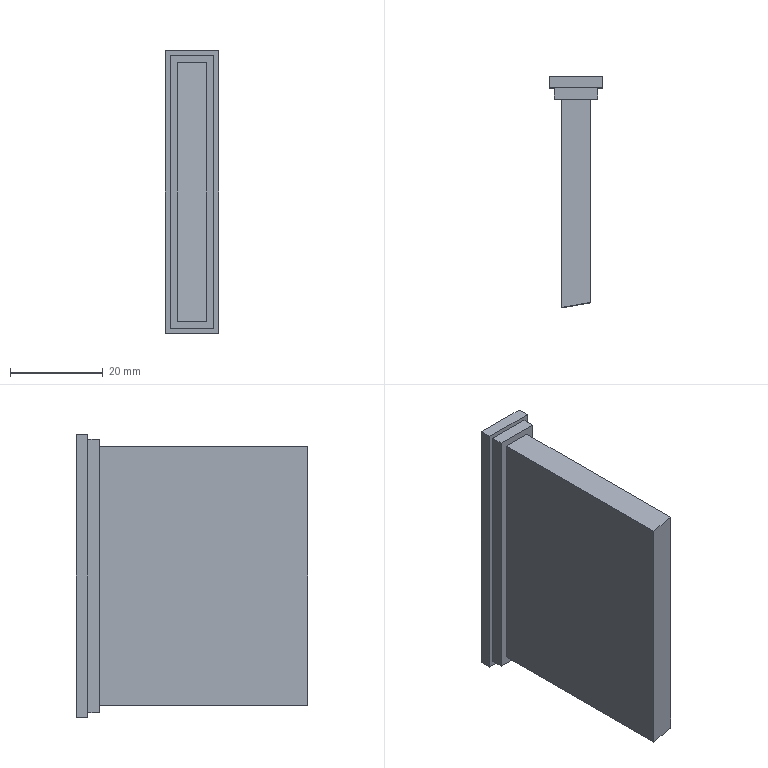Part | SolidWorks | features ICE 3, Extrusion 1 | 1 solid | 16 faces | box 11.5 x 50 x 61 mm | volume 18724 mm3 | plane 16
STEP:
#1=CARTESIAN_POINT('',(-3.14,0.,-27.89));
#2=VERTEX_POINT('',#1);
#3=CARTESIAN_POINT('',(-3.14,0.,27.89));
#4=VERTEX_POINT('',#3);
#5=CARTESIAN_POINT('',(-3.14,0.,-27.89));
#6=DIRECTION('',(0.,0.,1.));
#7=VECTOR('',#6,1000.);
#8=LINE('',#5,#7);
#9=EDGE_CURVE('',#2,#4,#8,.T.);
#10=ORIENTED_EDGE('',*,*,#9,.T.);
#11=CARTESIAN_POINT('',(-3.14,45.,27.89));
#12=VERTEX_POINT('',#11);
#13=CARTESIAN_POINT('',(-3.14,45.,27.89));
#14=DIRECTION('',(0.,-1.,0.));
#15=VECTOR('',#14,1000.);
#16=LINE('',#13,#15);
#17=EDGE_CURVE('',#12,#4,#16,.T.);
#18=ORIENTED_EDGE('',*,*,#17,.F.);
#19=CARTESIAN_POINT('',(-3.14,45.,-27.89));
#20=VERTEX_POINT('',#19);
#21=CARTESIAN_POINT('',(-3.14,45.,-27.89));
#22=DIRECTION('',(0.,0.,1.));
#23=VECTOR('',#22,1000.);
#24=LINE('',#21,#23);
#25=EDGE_CURVE('',#20,#12,#24,.T.);
#26=ORIENTED_EDGE('',*,*,#25,.F.);
#27=CARTESIAN_POINT('',(-3.14,45.,-27.89));
#28=DIRECTION('',(0.,-1.,0.));
#29=VECTOR('',#28,1000.);
#30=LINE('',#27,#29);
#31=EDGE_CURVE('',#20,#2,#30,.T.);
#32=ORIENTED_EDGE('',*,*,#31,.T.);
#33=EDGE_LOOP('',(#10,#18,#26,#32));
#34=FACE_OUTER_BOUND('',#33,.T.);
#35=CARTESIAN_POINT('',(-3.14,45.,-27.89));
#36=DIRECTION('',(1.,0.,0.));
#37=DIRECTION('',(0.,0.,-1.));
#38=AXIS2_PLACEMENT_3D('',#35,#36,#37);
#39=PLANE('',#38);
#40=ADVANCED_FACE('',(#34),#39,.F.);
#41=ORIENTED_EDGE('',*,*,#17,.T.);
#42=CARTESIAN_POINT('',(3.14,1.107,27.89));
#43=VERTEX_POINT('',#42);
#44=CARTESIAN_POINT('',(3.14,1.107,27.89));
#45=DIRECTION('',(-0.9848,-0.1736,0.));
#46=VECTOR('',#45,1000.);
#47=LINE('',#44,#46);
#48=EDGE_CURVE('',#43,#4,#47,.T.);
#49=ORIENTED_EDGE('',*,*,#48,.F.);
#50=CARTESIAN_POINT('',(3.14,45.,27.89));
#51=VERTEX_POINT('',#50);
#52=CARTESIAN_POINT('',(3.14,45.,27.89));
#53=DIRECTION('',(0.,-1.,0.));
#54=VECTOR('',#53,1000.);
#55=LINE('',#52,#54);
#56=EDGE_CURVE('',#51,#43,#55,.T.);
#57=ORIENTED_EDGE('',*,*,#56,.F.);
#58=CARTESIAN_POINT('',(-3.14,45.,27.89));
#59=DIRECTION('',(1.,0.,0.));
#60=VECTOR('',#59,1000.);
#61=LINE('',#58,#60);
#62=EDGE_CURVE('',#12,#51,#61,.T.);
#63=ORIENTED_EDGE('',*,*,#62,.F.);
#64=EDGE_LOOP('',(#41,#49,#57,#63));
#65=FACE_OUTER_BOUND('',#64,.T.);
#66=CARTESIAN_POINT('',(-3.14,45.,27.89));
#67=DIRECTION('',(0.,0.,-1.));
#68=DIRECTION('',(-1.,0.,0.));
#69=AXIS2_PLACEMENT_3D('',#66,#67,#68);
#70=PLANE('',#69);
#71=ADVANCED_FACE('',(#65),#70,.F.);
#72=ORIENTED_EDGE('',*,*,#56,.T.);
#73=CARTESIAN_POINT('',(3.14,1.107,-27.89));
#74=VERTEX_POINT('',#73);
#75=CARTESIAN_POINT('',(3.14,1.107,-27.89));
#76=DIRECTION('',(0.,0.,1.));
#77=VECTOR('',#76,1000.);
#78=LINE('',#75,#77);
#79=EDGE_CURVE('',#74,#43,#78,.T.);
#80=ORIENTED_EDGE('',*,*,#79,.F.);
#81=CARTESIAN_POINT('',(3.14,45.,-27.89));
#82=VERTEX_POINT('',#81);
#83=CARTESIAN_POINT('',(3.14,45.,-27.89));
#84=DIRECTION('',(0.,-1.,0.));
#85=VECTOR('',#84,1000.);
#86=LINE('',#83,#85);
#87=EDGE_CURVE('',#82,#74,#86,.T.);
#88=ORIENTED_EDGE('',*,*,#87,.F.);
#89=CARTESIAN_POINT('',(3.14,45.,-27.89));
#90=DIRECTION('',(0.,0.,-1.));
#91=VECTOR('',#90,1000.);
#92=LINE('',#89,#91);
#93=EDGE_CURVE('',#51,#82,#92,.T.);
#94=ORIENTED_EDGE('',*,*,#93,.F.);
#95=EDGE_LOOP('',(#72,#80,#88,#94));
#96=FACE_OUTER_BOUND('',#95,.T.);
#97=CARTESIAN_POINT('',(3.14,45.,-27.89));
#98=DIRECTION('',(-1.,0.,0.));
#99=DIRECTION('',(0.,0.,1.));
#100=AXIS2_PLACEMENT_3D('',#97,#98,#99);
#101=PLANE('',#100);
#102=ADVANCED_FACE('',(#96),#101,.F.);
#103=ORIENTED_EDGE('',*,*,#87,.T.);
#104=CARTESIAN_POINT('',(3.14,1.107,-27.89));
#105=DIRECTION('',(-0.9848,-0.1736,0.));
#106=VECTOR('',#105,1000.);
#107=LINE('',#104,#106);
#108=EDGE_CURVE('',#74,#2,#107,.T.);
#109=ORIENTED_EDGE('',*,*,#108,.T.);
#110=ORIENTED_EDGE('',*,*,#31,.F.);
#111=CARTESIAN_POINT('',(-3.14,45.,-27.89));
#112=DIRECTION('',(-1.,0.,0.));
#113=VECTOR('',#112,1000.);
#114=LINE('',#111,#113);
#115=EDGE_CURVE('',#82,#20,#114,.T.);
#116=ORIENTED_EDGE('',*,*,#115,.F.);
#117=EDGE_LOOP('',(#103,#109,#110,#116));
#118=FACE_OUTER_BOUND('',#117,.T.);
#119=CARTESIAN_POINT('',(-3.14,45.,-27.89));
#120=DIRECTION('',(0.,0.,1.));
#121=DIRECTION('',(1.,0.,0.));
#122=AXIS2_PLACEMENT_3D('',#119,#120,#121);
#123=PLANE('',#122);
#124=ADVANCED_FACE('',(#118),#123,.F.);
#125=ORIENTED_EDGE('',*,*,#48,.T.);
#126=ORIENTED_EDGE('',*,*,#9,.F.);
#127=ORIENTED_EDGE('',*,*,#108,.F.);
#128=ORIENTED_EDGE('',*,*,#79,.T.);
#129=EDGE_LOOP('',(#125,#126,#127,#128));
#130=FACE_OUTER_BOUND('',#129,.T.);
#131=CARTESIAN_POINT('',(3.14,1.107,-27.89));
#132=DIRECTION('',(-0.1736,0.9848,0.));
#133=DIRECTION('',(-0.9848,-0.1736,0.));
#134=AXIS2_PLACEMENT_3D('',#131,#132,#133);
#135=PLANE('',#134);
#136=ADVANCED_FACE('',(#130),#135,.F.);
#137=CARTESIAN_POINT('',(-4.75,45.,-29.5));
#138=VERTEX_POINT('',#137);
#139=CARTESIAN_POINT('',(-4.75,45.,29.5));
#140=VERTEX_POINT('',#139);
#141=CARTESIAN_POINT('',(-4.75,45.,-29.5));
#142=DIRECTION('',(0.,0.,1.));
#143=VECTOR('',#142,1000.);
#144=LINE('',#141,#143);
#145=EDGE_CURVE('',#138,#140,#144,.T.);
#146=ORIENTED_EDGE('',*,*,#145,.F.);
#147=CARTESIAN_POINT('',(4.75,45.,-29.5));
#148=VERTEX_POINT('',#147);
#149=CARTESIAN_POINT('',(-4.75,45.,-29.5));
#150=DIRECTION('',(-1.,0.,0.));
#151=VECTOR('',#150,1000.);
#152=LINE('',#149,#151);
#153=EDGE_CURVE('',#148,#138,#152,.T.);
#154=ORIENTED_EDGE('',*,*,#153,.F.);
#155=CARTESIAN_POINT('',(4.75,45.,29.5));
#156=VERTEX_POINT('',#155);
#157=CARTESIAN_POINT('',(4.75,45.,-29.5));
#158=DIRECTION('',(0.,0.,-1.));
#159=VECTOR('',#158,1000.);
#160=LINE('',#157,#159);
#161=EDGE_CURVE('',#156,#148,#160,.T.);
#162=ORIENTED_EDGE('',*,*,#161,.F.);
#163=CARTESIAN_POINT('',(-4.75,45.,29.5));
#164=DIRECTION('',(1.,0.,0.));
#165=VECTOR('',#164,1000.);
#166=LINE('',#163,#165);
#167=EDGE_CURVE('',#140,#156,#166,.T.);
#168=ORIENTED_EDGE('',*,*,#167,.F.);
#169=EDGE_LOOP('',(#146,#154,#162,#168));
#170=FACE_OUTER_BOUND('',#169,.T.);
#171=ORIENTED_EDGE('',*,*,#115,.T.);
#172=ORIENTED_EDGE('',*,*,#25,.T.);
#173=ORIENTED_EDGE('',*,*,#62,.T.);
#174=ORIENTED_EDGE('',*,*,#93,.T.);
#175=EDGE_LOOP('',(#171,#172,#173,#174));
#176=FACE_BOUND('',#175,.T.);
#177=CARTESIAN_POINT('',(0.,45.,0.));
#178=DIRECTION('',(0.,1.,0.));
#179=DIRECTION('',(0.,0.,1.));
#180=AXIS2_PLACEMENT_3D('',#177,#178,#179);
#181=PLANE('',#180);
#182=ADVANCED_FACE('',(#170,#176),#181,.F.);
#183=ORIENTED_EDGE('',*,*,#145,.T.);
#184=CARTESIAN_POINT('',(-4.75,47.5,29.5));
#185=VERTEX_POINT('',#184);
#186=CARTESIAN_POINT('',(-4.75,47.5,29.5));
#187=DIRECTION('',(0.,-1.,0.));
#188=VECTOR('',#187,1000.);
#189=LINE('',#186,#188);
#190=EDGE_CURVE('',#185,#140,#189,.T.);
#191=ORIENTED_EDGE('',*,*,#190,.F.);
#192=CARTESIAN_POINT('',(-4.75,47.5,-29.5));
#193=VERTEX_POINT('',#192);
#194=CARTESIAN_POINT('',(-4.75,47.5,-29.5));
#195=DIRECTION('',(0.,0.,1.));
#196=VECTOR('',#195,1000.);
#197=LINE('',#194,#196);
#198=EDGE_CURVE('',#193,#185,#197,.T.);
#199=ORIENTED_EDGE('',*,*,#198,.F.);
#200=CARTESIAN_POINT('',(-4.75,47.5,-29.5));
#201=DIRECTION('',(0.,-1.,0.));
#202=VECTOR('',#201,1000.);
#203=LINE('',#200,#202);
#204=EDGE_CURVE('',#193,#138,#203,.T.);
#205=ORIENTED_EDGE('',*,*,#204,.T.);
#206=EDGE_LOOP('',(#183,#191,#199,#205));
#207=FACE_OUTER_BOUND('',#206,.T.);
#208=CARTESIAN_POINT('',(-4.75,47.5,-29.5));
#209=DIRECTION('',(1.,0.,0.));
#210=DIRECTION('',(0.,0.,-1.));
#211=AXIS2_PLACEMENT_3D('',#208,#209,#210);
#212=PLANE('',#211);
#213=ADVANCED_FACE('',(#207),#212,.F.);
#214=ORIENTED_EDGE('',*,*,#167,.T.);
#215=CARTESIAN_POINT('',(4.75,47.5,29.5));
#216=VERTEX_POINT('',#215);
#217=CARTESIAN_POINT('',(4.75,47.5,29.5));
#218=DIRECTION('',(0.,-1.,0.));
#219=VECTOR('',#218,1000.);
#220=LINE('',#217,#219);
#221=EDGE_CURVE('',#216,#156,#220,.T.);
#222=ORIENTED_EDGE('',*,*,#221,.F.);
#223=CARTESIAN_POINT('',(-4.75,47.5,29.5));
#224=DIRECTION('',(1.,0.,0.));
#225=VECTOR('',#224,1000.);
#226=LINE('',#223,#225);
#227=EDGE_CURVE('',#185,#216,#226,.T.);
#228=ORIENTED_EDGE('',*,*,#227,.F.);
#229=ORIENTED_EDGE('',*,*,#190,.T.);
#230=EDGE_LOOP('',(#214,#222,#228,#229));
#231=FACE_OUTER_BOUND('',#230,.T.);
#232=CARTESIAN_POINT('',(-4.75,47.5,29.5));
#233=DIRECTION('',(0.,0.,-1.));
#234=DIRECTION('',(-1.,0.,0.));
#235=AXIS2_PLACEMENT_3D('',#232,#233,#234);
#236=PLANE('',#235);
#237=ADVANCED_FACE('',(#231),#236,.F.);
#238=ORIENTED_EDGE('',*,*,#161,.T.);
#239=CARTESIAN_POINT('',(4.75,47.5,-29.5));
#240=VERTEX_POINT('',#239);
#241=CARTESIAN_POINT('',(4.75,47.5,-29.5));
#242=DIRECTION('',(0.,-1.,0.));
#243=VECTOR('',#242,1000.);
#244=LINE('',#241,#243);
#245=EDGE_CURVE('',#240,#148,#244,.T.);
#246=ORIENTED_EDGE('',*,*,#245,.F.);
#247=CARTESIAN_POINT('',(4.75,47.5,-29.5));
#248=DIRECTION('',(0.,0.,-1.));
#249=VECTOR('',#248,1000.);
#250=LINE('',#247,#249);
#251=EDGE_CURVE('',#216,#240,#250,.T.);
#252=ORIENTED_EDGE('',*,*,#251,.F.);
#253=ORIENTED_EDGE('',*,*,#221,.T.);
#254=EDGE_LOOP('',(#238,#246,#252,#253));
#255=FACE_OUTER_BOUND('',#254,.T.);
#256=CARTESIAN_POINT('',(4.75,47.5,-29.5));
#257=DIRECTION('',(-1.,0.,0.));
#258=DIRECTION('',(0.,0.,1.));
#259=AXIS2_PLACEMENT_3D('',#256,#257,#258);
#260=PLANE('',#259);
#261=ADVANCED_FACE('',(#255),#260,.F.);
#262=ORIENTED_EDGE('',*,*,#153,.T.);
#263=ORIENTED_EDGE('',*,*,#204,.F.);
#264=CARTESIAN_POINT('',(-4.75,47.5,-29.5));
#265=DIRECTION('',(-1.,0.,0.));
#266=VECTOR('',#265,1000.);
#267=LINE('',#264,#266);
#268=EDGE_CURVE('',#240,#193,#267,.T.);
#269=ORIENTED_EDGE('',*,*,#268,.F.);
#270=ORIENTED_EDGE('',*,*,#245,.T.);
#271=EDGE_LOOP('',(#262,#263,#269,#270));
#272=FACE_OUTER_BOUND('',#271,.T.);
#273=CARTESIAN_POINT('',(-4.75,47.5,-29.5));
#274=DIRECTION('',(0.,0.,1.));
#275=DIRECTION('',(1.,0.,0.));
#276=AXIS2_PLACEMENT_3D('',#273,#274,#275);
#277=PLANE('',#276);
#278=ADVANCED_FACE('',(#272),#277,.F.);
#279=CARTESIAN_POINT('',(-5.75,47.5,-30.5));
#280=VERTEX_POINT('',#279);
#281=CARTESIAN_POINT('',(-5.75,47.5,30.5));
#282=VERTEX_POINT('',#281);
#283=CARTESIAN_POINT('',(-5.75,47.5,-30.5));
#284=DIRECTION('',(0.,0.,1.));
#285=VECTOR('',#284,1000.);
#286=LINE('',#283,#285);
#287=EDGE_CURVE('',#280,#282,#286,.T.);
#288=ORIENTED_EDGE('',*,*,#287,.F.);
#289=CARTESIAN_POINT('',(5.75,47.5,-30.5));
#290=VERTEX_POINT('',#289);
#291=CARTESIAN_POINT('',(-5.75,47.5,-30.5));
#292=DIRECTION('',(-1.,0.,0.));
#293=VECTOR('',#292,1000.);
#294=LINE('',#291,#293);
#295=EDGE_CURVE('',#290,#280,#294,.T.);
#296=ORIENTED_EDGE('',*,*,#295,.F.);
#297=CARTESIAN_POINT('',(5.75,47.5,30.5));
#298=VERTEX_POINT('',#297);
#299=CARTESIAN_POINT('',(5.75,47.5,-30.5));
#300=DIRECTION('',(0.,0.,-1.));
#301=VECTOR('',#300,1000.);
#302=LINE('',#299,#301);
#303=EDGE_CURVE('',#298,#290,#302,.T.);
#304=ORIENTED_EDGE('',*,*,#303,.F.);
#305=CARTESIAN_POINT('',(-5.75,47.5,30.5));
#306=DIRECTION('',(1.,0.,0.));
#307=VECTOR('',#306,1000.);
#308=LINE('',#305,#307);
#309=EDGE_CURVE('',#282,#298,#308,.T.);
#310=ORIENTED_EDGE('',*,*,#309,.F.);
#311=EDGE_LOOP('',(#288,#296,#304,#310));
#312=FACE_OUTER_BOUND('',#311,.T.);
#313=ORIENTED_EDGE('',*,*,#268,.T.);
#314=ORIENTED_EDGE('',*,*,#198,.T.);
#315=ORIENTED_EDGE('',*,*,#227,.T.);
#316=ORIENTED_EDGE('',*,*,#251,.T.);
#317=EDGE_LOOP('',(#313,#314,#315,#316));
#318=FACE_BOUND('',#317,.T.);
#319=CARTESIAN_POINT('',(0.,47.5,0.));
#320=DIRECTION('',(0.,1.,0.));
#321=DIRECTION('',(0.,0.,1.));
#322=AXIS2_PLACEMENT_3D('',#319,#320,#321);
#323=PLANE('',#322);
#324=ADVANCED_FACE('',(#312,#318),#323,.F.);
#325=ORIENTED_EDGE('',*,*,#287,.T.);
#326=CARTESIAN_POINT('',(-5.75,50.,30.5));
#327=VERTEX_POINT('',#326);
#328=CARTESIAN_POINT('',(-5.75,50.,30.5));
#329=DIRECTION('',(0.,-1.,0.));
#330=VECTOR('',#329,1000.);
#331=LINE('',#328,#330);
#332=EDGE_CURVE('',#327,#282,#331,.T.);
#333=ORIENTED_EDGE('',*,*,#332,.F.);
#334=CARTESIAN_POINT('',(-5.75,50.,-30.5));
#335=VERTEX_POINT('',#334);
#336=CARTESIAN_POINT('',(-5.75,50.,-30.5));
#337=DIRECTION('',(0.,0.,1.));
#338=VECTOR('',#337,1000.);
#339=LINE('',#336,#338);
#340=EDGE_CURVE('',#335,#327,#339,.T.);
#341=ORIENTED_EDGE('',*,*,#340,.F.);
#342=CARTESIAN_POINT('',(-5.75,50.,-30.5));
#343=DIRECTION('',(0.,-1.,0.));
#344=VECTOR('',#343,1000.);
#345=LINE('',#342,#344);
#346=EDGE_CURVE('',#335,#280,#345,.T.);
#347=ORIENTED_EDGE('',*,*,#346,.T.);
#348=EDGE_LOOP('',(#325,#333,#341,#347));
#349=FACE_OUTER_BOUND('',#348,.T.);
#350=CARTESIAN_POINT('',(-5.75,50.,-30.5));
#351=DIRECTION('',(1.,0.,0.));
#352=DIRECTION('',(0.,0.,-1.));
#353=AXIS2_PLACEMENT_3D('',#350,#351,#352);
#354=PLANE('',#353);
#355=ADVANCED_FACE('',(#349),#354,.F.);
#356=ORIENTED_EDGE('',*,*,#309,.T.);
#357=CARTESIAN_POINT('',(5.75,50.,30.5));
#358=VERTEX_POINT('',#357);
#359=CARTESIAN_POINT('',(5.75,50.,30.5));
#360=DIRECTION('',(0.,-1.,0.));
#361=VECTOR('',#360,1000.);
#362=LINE('',#359,#361);
#363=EDGE_CURVE('',#358,#298,#362,.T.);
#364=ORIENTED_EDGE('',*,*,#363,.F.);
#365=CARTESIAN_POINT('',(-5.75,50.,30.5));
#366=DIRECTION('',(1.,0.,0.));
#367=VECTOR('',#366,1000.);
#368=LINE('',#365,#367);
#369=EDGE_CURVE('',#327,#358,#368,.T.);
#370=ORIENTED_EDGE('',*,*,#369,.F.);
#371=ORIENTED_EDGE('',*,*,#332,.T.);
#372=EDGE_LOOP('',(#356,#364,#370,#371));
#373=FACE_OUTER_BOUND('',#372,.T.);
#374=CARTESIAN_POINT('',(-5.75,50.,30.5));
#375=DIRECTION('',(0.,0.,-1.));
#376=DIRECTION('',(-1.,0.,0.));
#377=AXIS2_PLACEMENT_3D('',#374,#375,#376);
#378=PLANE('',#377);
#379=ADVANCED_FACE('',(#373),#378,.F.);
#380=ORIENTED_EDGE('',*,*,#303,.T.);
#381=CARTESIAN_POINT('',(5.75,50.,-30.5));
#382=VERTEX_POINT('',#381);
#383=CARTESIAN_POINT('',(5.75,50.,-30.5));
#384=DIRECTION('',(0.,-1.,0.));
#385=VECTOR('',#384,1000.);
#386=LINE('',#383,#385);
#387=EDGE_CURVE('',#382,#290,#386,.T.);
#388=ORIENTED_EDGE('',*,*,#387,.F.);
#389=CARTESIAN_POINT('',(5.75,50.,-30.5));
#390=DIRECTION('',(0.,0.,-1.));
#391=VECTOR('',#390,1000.);
#392=LINE('',#389,#391);
#393=EDGE_CURVE('',#358,#382,#392,.T.);
#394=ORIENTED_EDGE('',*,*,#393,.F.);
#395=ORIENTED_EDGE('',*,*,#363,.T.);
#396=EDGE_LOOP('',(#380,#388,#394,#395));
#397=FACE_OUTER_BOUND('',#396,.T.);
#398=CARTESIAN_POINT('',(5.75,50.,-30.5));
#399=DIRECTION('',(-1.,0.,0.));
#400=DIRECTION('',(0.,0.,1.));
#401=AXIS2_PLACEMENT_3D('',#398,#399,#400);
#402=PLANE('',#401);
#403=ADVANCED_FACE('',(#397),#402,.F.);
#404=ORIENTED_EDGE('',*,*,#295,.T.);
#405=ORIENTED_EDGE('',*,*,#346,.F.);
#406=CARTESIAN_POINT('',(-5.75,50.,-30.5));
#407=DIRECTION('',(-1.,0.,0.));
#408=VECTOR('',#407,1000.);
#409=LINE('',#406,#408);
#410=EDGE_CURVE('',#382,#335,#409,.T.);
#411=ORIENTED_EDGE('',*,*,#410,.F.);
#412=ORIENTED_EDGE('',*,*,#387,.T.);
#413=EDGE_LOOP('',(#404,#405,#411,#412));
#414=FACE_OUTER_BOUND('',#413,.T.);
#415=CARTESIAN_POINT('',(-5.75,50.,-30.5));
#416=DIRECTION('',(0.,0.,1.));
#417=DIRECTION('',(1.,0.,0.));
#418=AXIS2_PLACEMENT_3D('',#415,#416,#417);
#419=PLANE('',#418);
#420=ADVANCED_FACE('',(#414),#419,.F.);
#421=ORIENTED_EDGE('',*,*,#340,.T.);
#422=ORIENTED_EDGE('',*,*,#369,.T.);
#423=ORIENTED_EDGE('',*,*,#393,.T.);
#424=ORIENTED_EDGE('',*,*,#410,.T.);
#425=EDGE_LOOP('',(#421,#422,#423,#424));
#426=FACE_OUTER_BOUND('',#425,.T.);
#427=CARTESIAN_POINT('',(0.,50.,0.));
#428=DIRECTION('',(0.,1.,0.));
#429=DIRECTION('',(0.,0.,1.));
#430=AXIS2_PLACEMENT_3D('',#427,#428,#429);
#431=PLANE('',#430);
#432=ADVANCED_FACE('',(#426),#431,.T.);
#433=CLOSED_SHELL('',(#40,#71,#102,#124,#136,#182,#213,#237,#261,#278,#324,#355,#379,#403,#420,#432));
#434=MANIFOLD_SOLID_BREP('',#433);
#435=CARTESIAN_POINT('',(0.,0.,0.));
#436=DIRECTION('',(0.,0.,1.));
#437=DIRECTION('',(1.,0.,0.));
#438=AXIS2_PLACEMENT_3D('',#435,#436,#437);
#439=(LENGTH_UNIT()NAMED_UNIT(*)SI_UNIT(.MILLI.,.METRE.));
#440=UNCERTAINTY_MEASURE_WITH_UNIT(LENGTH_MEASURE(0.00001),#439,'','');
#441=(NAMED_UNIT(*)PLANE_ANGLE_UNIT()SI_UNIT($,.RADIAN.));
#442=(NAMED_UNIT(*)SI_UNIT($,.STERADIAN.)SOLID_ANGLE_UNIT());
#443=(GEOMETRIC_REPRESENTATION_CONTEXT(3)GLOBAL_UNCERTAINTY_ASSIGNED_CONTEXT((#440))GLOBAL_UNIT_ASSIGNED_CONTEXT((#439,#441,#442))REPRESENTATION_CONTEXT('',''));
#444=ADVANCED_BREP_SHAPE_REPRESENTATION('',(#434,#438),#443);